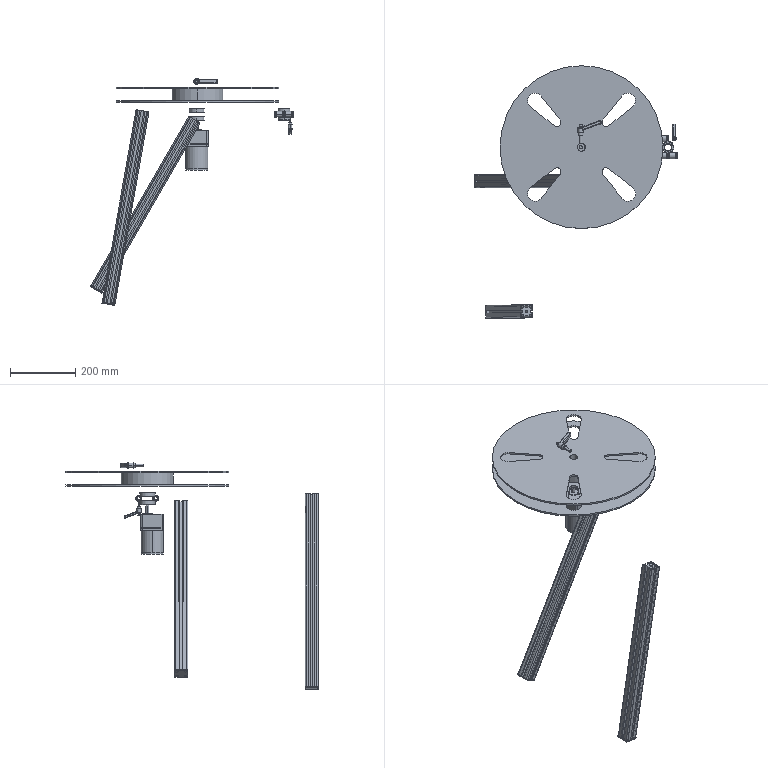Part | NX | 15 solids | 675 faces | box 622.817 x 774 x 696.596 mm | volume 4156416 mm3 | cylinder 260 | plane 258 | cone 68 | torus 57 | spline 22 | sphere 10 | commonest cylinder face diameters 8 x34 10 x18 19 x18 25 x18 1 x16 5.5 x16